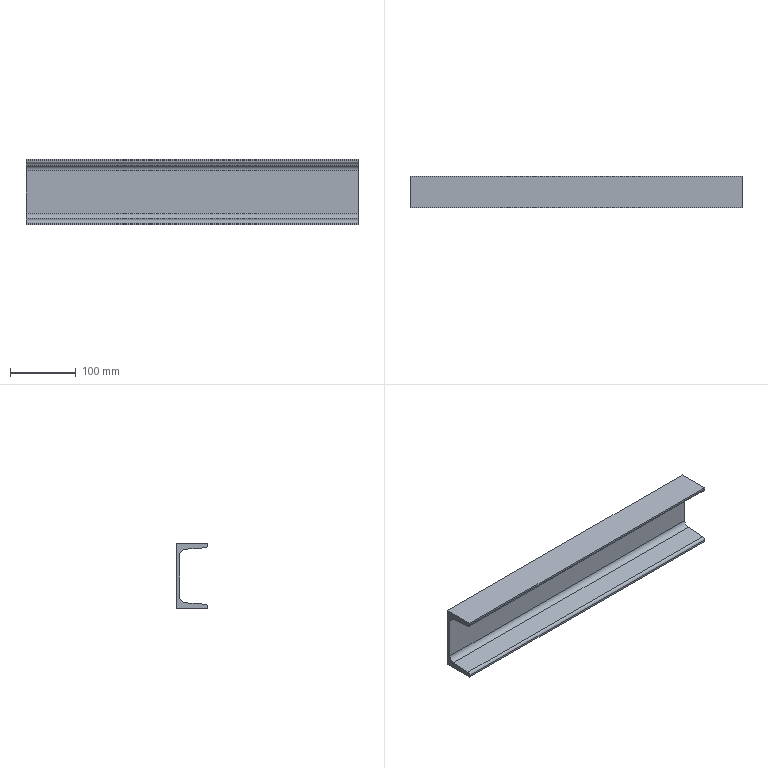Part | STEP file | 02-Channel 100x48_default<machining> | 1 solid | 14 faces | box 505 x 48 x 100 mm | volume 635347 mm3 | plane 10 | cylinder 4 | commonest cylinder face diameters 8.5 x2 17 x2
STEP:
#1=CARTESIAN_POINT('',(0.,0.,0.));
#2=DIRECTION('',(0.,0.,1.));
#3=DIRECTION('',(1.,0.,0.));
#4=AXIS2_PLACEMENT_3D('',#1,#2,#3);
#5=CARTESIAN_POINT('',(0.,-48.,-100.));
#6=VERTEX_POINT('',#5);
#7=CARTESIAN_POINT('',(0.,0.,-100.));
#8=VERTEX_POINT('',#7);
#9=CARTESIAN_POINT('',(0.,0.,-100.));
#10=DIRECTION('',(0.,1.,0.));
#11=VECTOR('',#10,1.);
#12=LINE('',#9,#11);
#13=CARTESIAN_POINT('',(505.,0.,-100.));
#14=DIRECTION('',(0.,0.,1.));
#15=DIRECTION('',(1.,0.,0.));
#16=AXIS2_PLACEMENT_3D('',#13,#14,#15);
#17=PLANE('',#16);
#18=CARTESIAN_POINT('',(-505.,0.));
#19=DIRECTION('',(0.,1.));
#20=VECTOR('',#19,1.);
#21=LINE('',#18,#20);
#22=(GEOMETRIC_REPRESENTATION_CONTEXT(2)PARAMETRIC_REPRESENTATION_CONTEXT()REPRESENTATION_CONTEXT('',''));
#23=DEFINITIONAL_REPRESENTATION('',(#21),#22);
#24=PCURVE('',#17,#23);
#25=CARTESIAN_POINT('',(0.,-43.75,-97.266));
#26=DIRECTION('',(1.,0.,0.));
#27=DIRECTION('',(0.,0.,-1.));
#28=AXIS2_PLACEMENT_3D('',#25,#26,#27);
#29=PLANE('',#28);
#30=CARTESIAN_POINT('',(2.734,43.75));
#31=DIRECTION('',(0.,1.));
#32=VECTOR('',#31,1.);
#33=LINE('',#30,#32);
#34=(GEOMETRIC_REPRESENTATION_CONTEXT(2)PARAMETRIC_REPRESENTATION_CONTEXT()REPRESENTATION_CONTEXT('',''));
#35=DEFINITIONAL_REPRESENTATION('',(#33),#34);
#36=PCURVE('',#29,#35);
#37=SURFACE_CURVE('',#12,(#24,#36),.PCURVE_S1.);
#38=EDGE_CURVE('',#6,#8,#37,.T.);
#39=ORIENTED_EDGE('',*,*,#38,.T.);
#40=CARTESIAN_POINT('',(505.,0.,-100.));
#41=VERTEX_POINT('',#40);
#42=CARTESIAN_POINT('',(505.,0.,-100.));
#43=DIRECTION('',(-1.,0.,0.));
#44=VECTOR('',#43,1.);
#45=LINE('',#42,#44);
#46=CARTESIAN_POINT('',(0.,0.));
#47=DIRECTION('',(-1.,0.));
#48=VECTOR('',#47,1.);
#49=LINE('',#46,#48);
#50=(GEOMETRIC_REPRESENTATION_CONTEXT(2)PARAMETRIC_REPRESENTATION_CONTEXT()REPRESENTATION_CONTEXT('',''));
#51=DEFINITIONAL_REPRESENTATION('',(#49),#50);
#52=PCURVE('',#17,#51);
#53=CARTESIAN_POINT('',(505.,0.,0.));
#54=DIRECTION('',(0.,-1.,0.));
#55=DIRECTION('',(0.,0.,-1.));
#56=AXIS2_PLACEMENT_3D('',#53,#54,#55);
#57=PLANE('',#56);
#58=CARTESIAN_POINT('',(100.,0.));
#59=DIRECTION('',(0.,-1.));
#60=VECTOR('',#59,1.);
#61=LINE('',#58,#60);
#62=(GEOMETRIC_REPRESENTATION_CONTEXT(2)PARAMETRIC_REPRESENTATION_CONTEXT()REPRESENTATION_CONTEXT('',''));
#63=DEFINITIONAL_REPRESENTATION('',(#61),#62);
#64=PCURVE('',#57,#63);
#65=SURFACE_CURVE('',#45,(#52,#64),.PCURVE_S1.);
#66=EDGE_CURVE('',#41,#8,#65,.T.);
#67=ORIENTED_EDGE('',*,*,#66,.F.);
#68=CARTESIAN_POINT('',(505.,-48.,-100.));
#69=VERTEX_POINT('',#68);
#70=CARTESIAN_POINT('',(505.,0.,-100.));
#71=DIRECTION('',(0.,1.,0.));
#72=VECTOR('',#71,1.);
#73=LINE('',#70,#72);
#74=CARTESIAN_POINT('',(0.,0.));
#75=DIRECTION('',(0.,1.));
#76=VECTOR('',#75,1.);
#77=LINE('',#74,#76);
#78=(GEOMETRIC_REPRESENTATION_CONTEXT(2)PARAMETRIC_REPRESENTATION_CONTEXT()REPRESENTATION_CONTEXT('',''));
#79=DEFINITIONAL_REPRESENTATION('',(#77),#78);
#80=PCURVE('',#17,#79);
#81=CARTESIAN_POINT('',(505.,-43.75,-97.266));
#82=DIRECTION('',(1.,0.,0.));
#83=DIRECTION('',(0.,0.,-1.));
#84=AXIS2_PLACEMENT_3D('',#81,#82,#83);
#85=PLANE('',#84);
#86=CARTESIAN_POINT('',(2.734,43.75));
#87=DIRECTION('',(0.,1.));
#88=VECTOR('',#87,1.);
#89=LINE('',#86,#88);
#90=(GEOMETRIC_REPRESENTATION_CONTEXT(2)PARAMETRIC_REPRESENTATION_CONTEXT()REPRESENTATION_CONTEXT('',''));
#91=DEFINITIONAL_REPRESENTATION('',(#89),#90);
#92=PCURVE('',#85,#91);
#93=SURFACE_CURVE('',#73,(#80,#92),.PCURVE_S1.);
#94=EDGE_CURVE('',#69,#41,#93,.T.);
#95=ORIENTED_EDGE('',*,*,#94,.F.);
#96=CARTESIAN_POINT('',(505.,-48.,-100.));
#97=DIRECTION('',(-1.,0.,0.));
#98=VECTOR('',#97,1.);
#99=LINE('',#96,#98);
#100=CARTESIAN_POINT('',(0.,-48.));
#101=DIRECTION('',(-1.,0.));
#102=VECTOR('',#101,1.);
#103=LINE('',#100,#102);
#104=(GEOMETRIC_REPRESENTATION_CONTEXT(2)PARAMETRIC_REPRESENTATION_CONTEXT()REPRESENTATION_CONTEXT('',''));
#105=DEFINITIONAL_REPRESENTATION('',(#103),#104);
#106=PCURVE('',#17,#105);
#107=CARTESIAN_POINT('',(505.,-48.,-97.266));
#108=DIRECTION('',(0.,1.,0.));
#109=DIRECTION('',(0.,0.,1.));
#110=AXIS2_PLACEMENT_3D('',#107,#108,#109);
#111=PLANE('',#110);
#112=CARTESIAN_POINT('',(-2.734,0.));
#113=DIRECTION('',(0.,-1.));
#114=VECTOR('',#113,1.);
#115=LINE('',#112,#114);
#116=(GEOMETRIC_REPRESENTATION_CONTEXT(2)PARAMETRIC_REPRESENTATION_CONTEXT()REPRESENTATION_CONTEXT('',''));
#117=DEFINITIONAL_REPRESENTATION('',(#115),#116);
#118=PCURVE('',#111,#117);
#119=SURFACE_CURVE('',#99,(#106,#118),.PCURVE_S1.);
#120=EDGE_CURVE('',#69,#6,#119,.T.);
#121=ORIENTED_EDGE('',*,*,#120,.T.);
#122=EDGE_LOOP('',(#39,#67,#95,#121));
#123=FACE_BOUND('',#122,.T.);
#124=ADVANCED_FACE('',(#123),#17,.F.);
#125=CARTESIAN_POINT('',(0.,0.,0.));
#126=VERTEX_POINT('',#125);
#127=CARTESIAN_POINT('',(0.,0.,0.));
#128=DIRECTION('',(0.,0.,1.));
#129=VECTOR('',#128,1.);
#130=LINE('',#127,#129);
#131=CARTESIAN_POINT('',(0.,-505.));
#132=DIRECTION('',(-1.,0.));
#133=VECTOR('',#132,1.);
#134=LINE('',#131,#133);
#135=(GEOMETRIC_REPRESENTATION_CONTEXT(2)PARAMETRIC_REPRESENTATION_CONTEXT()REPRESENTATION_CONTEXT('',''));
#136=DEFINITIONAL_REPRESENTATION('',(#134),#135);
#137=PCURVE('',#57,#136);
#138=CARTESIAN_POINT('',(-97.266,43.75));
#139=DIRECTION('',(-1.,0.));
#140=VECTOR('',#139,1.);
#141=LINE('',#138,#140);
#142=(GEOMETRIC_REPRESENTATION_CONTEXT(2)PARAMETRIC_REPRESENTATION_CONTEXT()REPRESENTATION_CONTEXT('',''));
#143=DEFINITIONAL_REPRESENTATION('',(#141),#142);
#144=PCURVE('',#29,#143);
#145=SURFACE_CURVE('',#130,(#137,#144),.PCURVE_S1.);
#146=EDGE_CURVE('',#8,#126,#145,.T.);
#147=ORIENTED_EDGE('',*,*,#146,.T.);
#148=CARTESIAN_POINT('',(505.,0.,0.));
#149=VERTEX_POINT('',#148);
#150=CARTESIAN_POINT('',(505.,0.,0.));
#151=DIRECTION('',(-1.,0.,0.));
#152=VECTOR('',#151,1.);
#153=LINE('',#150,#152);
#154=CARTESIAN_POINT('',(0.,0.));
#155=DIRECTION('',(0.,-1.));
#156=VECTOR('',#155,1.);
#157=LINE('',#154,#156);
#158=(GEOMETRIC_REPRESENTATION_CONTEXT(2)PARAMETRIC_REPRESENTATION_CONTEXT()REPRESENTATION_CONTEXT('',''));
#159=DEFINITIONAL_REPRESENTATION('',(#157),#158);
#160=PCURVE('',#57,#159);
#161=CARTESIAN_POINT('',(505.,0.,0.));
#162=DIRECTION('',(0.,0.,-1.));
#163=DIRECTION('',(0.,1.,0.));
#164=AXIS2_PLACEMENT_3D('',#161,#162,#163);
#165=PLANE('',#164);
#166=CARTESIAN_POINT('',(0.,0.));
#167=DIRECTION('',(0.,-1.));
#168=VECTOR('',#167,1.);
#169=LINE('',#166,#168);
#170=(GEOMETRIC_REPRESENTATION_CONTEXT(2)PARAMETRIC_REPRESENTATION_CONTEXT()REPRESENTATION_CONTEXT('',''));
#171=DEFINITIONAL_REPRESENTATION('',(#169),#170);
#172=PCURVE('',#165,#171);
#173=SURFACE_CURVE('',#153,(#160,#172),.PCURVE_S1.);
#174=EDGE_CURVE('',#149,#126,#173,.T.);
#175=ORIENTED_EDGE('',*,*,#174,.F.);
#176=CARTESIAN_POINT('',(505.,0.,0.));
#177=DIRECTION('',(0.,0.,1.));
#178=VECTOR('',#177,1.);
#179=LINE('',#176,#178);
#180=CARTESIAN_POINT('',(0.,0.));
#181=DIRECTION('',(-1.,0.));
#182=VECTOR('',#181,1.);
#183=LINE('',#180,#182);
#184=(GEOMETRIC_REPRESENTATION_CONTEXT(2)PARAMETRIC_REPRESENTATION_CONTEXT()REPRESENTATION_CONTEXT('',''));
#185=DEFINITIONAL_REPRESENTATION('',(#183),#184);
#186=PCURVE('',#57,#185);
#187=CARTESIAN_POINT('',(-97.266,43.75));
#188=DIRECTION('',(-1.,0.));
#189=VECTOR('',#188,1.);
#190=LINE('',#187,#189);
#191=(GEOMETRIC_REPRESENTATION_CONTEXT(2)PARAMETRIC_REPRESENTATION_CONTEXT()REPRESENTATION_CONTEXT('',''));
#192=DEFINITIONAL_REPRESENTATION('',(#190),#191);
#193=PCURVE('',#85,#192);
#194=SURFACE_CURVE('',#179,(#186,#193),.PCURVE_S1.);
#195=EDGE_CURVE('',#41,#149,#194,.T.);
#196=ORIENTED_EDGE('',*,*,#195,.F.);
#197=ORIENTED_EDGE('',*,*,#66,.T.);
#198=EDGE_LOOP('',(#147,#175,#196,#197));
#199=FACE_BOUND('',#198,.T.);
#200=ADVANCED_FACE('',(#199),#57,.F.);
#201=CARTESIAN_POINT('',(0.,-48.,0.));
#202=VERTEX_POINT('',#201);
#203=CARTESIAN_POINT('',(0.,0.,0.));
#204=DIRECTION('',(0.,-1.,0.));
#205=VECTOR('',#204,1.);
#206=LINE('',#203,#205);
#207=CARTESIAN_POINT('',(0.,-505.));
#208=DIRECTION('',(-1.,0.));
#209=VECTOR('',#208,1.);
#210=LINE('',#207,#209);
#211=(GEOMETRIC_REPRESENTATION_CONTEXT(2)PARAMETRIC_REPRESENTATION_CONTEXT()REPRESENTATION_CONTEXT('',''));
#212=DEFINITIONAL_REPRESENTATION('',(#210),#211);
#213=PCURVE('',#165,#212);
#214=CARTESIAN_POINT('',(-97.266,43.75));
#215=DIRECTION('',(0.,-1.));
#216=VECTOR('',#215,1.);
#217=LINE('',#214,#216);
#218=(GEOMETRIC_REPRESENTATION_CONTEXT(2)PARAMETRIC_REPRESENTATION_CONTEXT()REPRESENTATION_CONTEXT('',''));
#219=DEFINITIONAL_REPRESENTATION('',(#217),#218);
#220=PCURVE('',#29,#219);
#221=SURFACE_CURVE('',#206,(#213,#220),.PCURVE_S1.);
#222=EDGE_CURVE('',#126,#202,#221,.T.);
#223=ORIENTED_EDGE('',*,*,#222,.T.);
#224=CARTESIAN_POINT('',(505.,-48.,0.));
#225=VERTEX_POINT('',#224);
#226=CARTESIAN_POINT('',(505.,-48.,0.));
#227=DIRECTION('',(-1.,0.,0.));
#228=VECTOR('',#227,1.);
#229=LINE('',#226,#228);
#230=CARTESIAN_POINT('',(-48.,0.));
#231=DIRECTION('',(0.,-1.));
#232=VECTOR('',#231,1.);
#233=LINE('',#230,#232);
#234=(GEOMETRIC_REPRESENTATION_CONTEXT(2)PARAMETRIC_REPRESENTATION_CONTEXT()REPRESENTATION_CONTEXT('',''));
#235=DEFINITIONAL_REPRESENTATION('',(#233),#234);
#236=PCURVE('',#165,#235);
#237=CARTESIAN_POINT('',(505.,-48.,-2.734));
#238=DIRECTION('',(0.,1.,0.));
#239=DIRECTION('',(0.,0.,1.));
#240=AXIS2_PLACEMENT_3D('',#237,#238,#239);
#241=PLANE('',#240);
#242=CARTESIAN_POINT('',(2.734,0.));
#243=DIRECTION('',(0.,-1.));
#244=VECTOR('',#243,1.);
#245=LINE('',#242,#244);
#246=(GEOMETRIC_REPRESENTATION_CONTEXT(2)PARAMETRIC_REPRESENTATION_CONTEXT()REPRESENTATION_CONTEXT('',''));
#247=DEFINITIONAL_REPRESENTATION('',(#245),#246);
#248=PCURVE('',#241,#247);
#249=SURFACE_CURVE('',#229,(#236,#248),.PCURVE_S1.);
#250=EDGE_CURVE('',#225,#202,#249,.T.);
#251=ORIENTED_EDGE('',*,*,#250,.F.);
#252=CARTESIAN_POINT('',(505.,0.,0.));
#253=DIRECTION('',(0.,-1.,0.));
#254=VECTOR('',#253,1.);
#255=LINE('',#252,#254);
#256=CARTESIAN_POINT('',(0.,0.));
#257=DIRECTION('',(-1.,0.));
#258=VECTOR('',#257,1.);
#259=LINE('',#256,#258);
#260=(GEOMETRIC_REPRESENTATION_CONTEXT(2)PARAMETRIC_REPRESENTATION_CONTEXT()REPRESENTATION_CONTEXT('',''));
#261=DEFINITIONAL_REPRESENTATION('',(#259),#260);
#262=PCURVE('',#165,#261);
#263=CARTESIAN_POINT('',(-97.266,43.75));
#264=DIRECTION('',(0.,-1.));
#265=VECTOR('',#264,1.);
#266=LINE('',#263,#265);
#267=(GEOMETRIC_REPRESENTATION_CONTEXT(2)PARAMETRIC_REPRESENTATION_CONTEXT()REPRESENTATION_CONTEXT('',''));
#268=DEFINITIONAL_REPRESENTATION('',(#266),#267);
#269=PCURVE('',#85,#268);
#270=SURFACE_CURVE('',#255,(#262,#269),.PCURVE_S1.);
#271=EDGE_CURVE('',#149,#225,#270,.T.);
#272=ORIENTED_EDGE('',*,*,#271,.F.);
#273=ORIENTED_EDGE('',*,*,#174,.T.);
#274=EDGE_LOOP('',(#223,#251,#272,#273));
#275=FACE_BOUND('',#274,.T.);
#276=ADVANCED_FACE('',(#275),#165,.F.);
#277=CARTESIAN_POINT('',(0.,-48.,-2.734));
#278=VERTEX_POINT('',#277);
#279=CARTESIAN_POINT('',(0.,-48.,-2.734));
#280=DIRECTION('',(0.,0.,-1.));
#281=VECTOR('',#280,1.);
#282=LINE('',#279,#281);
#283=CARTESIAN_POINT('',(0.,-505.));
#284=DIRECTION('',(-1.,0.));
#285=VECTOR('',#284,1.);
#286=LINE('',#283,#285);
#287=(GEOMETRIC_REPRESENTATION_CONTEXT(2)PARAMETRIC_REPRESENTATION_CONTEXT()REPRESENTATION_CONTEXT('',''));
#288=DEFINITIONAL_REPRESENTATION('',(#286),#287);
#289=PCURVE('',#241,#288);
#290=CARTESIAN_POINT('',(-94.531,-4.25));
#291=DIRECTION('',(1.,0.));
#292=VECTOR('',#291,1.);
#293=LINE('',#290,#292);
#294=(GEOMETRIC_REPRESENTATION_CONTEXT(2)PARAMETRIC_REPRESENTATION_CONTEXT()REPRESENTATION_CONTEXT('',''));
#295=DEFINITIONAL_REPRESENTATION('',(#293),#294);
#296=PCURVE('',#29,#295);
#297=SURFACE_CURVE('',#282,(#289,#296),.PCURVE_S1.);
#298=EDGE_CURVE('',#202,#278,#297,.T.);
#299=ORIENTED_EDGE('',*,*,#298,.T.);
#300=CARTESIAN_POINT('',(505.,-48.,-2.734));
#301=VERTEX_POINT('',#300);
#302=CARTESIAN_POINT('',(505.,-48.,-2.734));
#303=DIRECTION('',(-1.,0.,0.));
#304=VECTOR('',#303,1.);
#305=LINE('',#302,#304);
#306=CARTESIAN_POINT('',(0.,0.));
#307=DIRECTION('',(0.,-1.));
#308=VECTOR('',#307,1.);
#309=LINE('',#306,#308);
#310=(GEOMETRIC_REPRESENTATION_CONTEXT(2)PARAMETRIC_REPRESENTATION_CONTEXT()REPRESENTATION_CONTEXT('',''));
#311=DEFINITIONAL_REPRESENTATION('',(#309),#310);
#312=PCURVE('',#241,#311);
#313=CARTESIAN_POINT('',(505.,-43.75,-2.734));
#314=DIRECTION('',(-1.,0.,0.));
#315=DIRECTION('',(0.,0.,1.));
#316=AXIS2_PLACEMENT_3D('',#313,#314,#315);
#317=CYLINDRICAL_SURFACE('',#316,4.25);
#318=CARTESIAN_POINT('',(4.712,0.));
#319=DIRECTION('',(0.,1.));
#320=VECTOR('',#319,1.);
#321=LINE('',#318,#320);
#322=(GEOMETRIC_REPRESENTATION_CONTEXT(2)PARAMETRIC_REPRESENTATION_CONTEXT()REPRESENTATION_CONTEXT('',''));
#323=DEFINITIONAL_REPRESENTATION('',(#321),#322);
#324=PCURVE('',#317,#323);
#325=SURFACE_CURVE('',#305,(#312,#324),.PCURVE_S1.);
#326=EDGE_CURVE('',#301,#278,#325,.T.);
#327=ORIENTED_EDGE('',*,*,#326,.F.);
#328=CARTESIAN_POINT('',(505.,-48.,-2.734));
#329=DIRECTION('',(0.,0.,-1.));
#330=VECTOR('',#329,1.);
#331=LINE('',#328,#330);
#332=CARTESIAN_POINT('',(0.,0.));
#333=DIRECTION('',(-1.,0.));
#334=VECTOR('',#333,1.);
#335=LINE('',#332,#334);
#336=(GEOMETRIC_REPRESENTATION_CONTEXT(2)PARAMETRIC_REPRESENTATION_CONTEXT()REPRESENTATION_CONTEXT('',''));
#337=DEFINITIONAL_REPRESENTATION('',(#335),#336);
#338=PCURVE('',#241,#337);
#339=CARTESIAN_POINT('',(-94.531,-4.25));
#340=DIRECTION('',(1.,0.));
#341=VECTOR('',#340,1.);
#342=LINE('',#339,#341);
#343=(GEOMETRIC_REPRESENTATION_CONTEXT(2)PARAMETRIC_REPRESENTATION_CONTEXT()REPRESENTATION_CONTEXT('',''));
#344=DEFINITIONAL_REPRESENTATION('',(#342),#343);
#345=PCURVE('',#85,#344);
#346=SURFACE_CURVE('',#331,(#338,#345),.PCURVE_S1.);
#347=EDGE_CURVE('',#225,#301,#346,.T.);
#348=ORIENTED_EDGE('',*,*,#347,.F.);
#349=ORIENTED_EDGE('',*,*,#250,.T.);
#350=EDGE_LOOP('',(#299,#327,#348,#349));
#351=FACE_BOUND('',#350,.T.);
#352=ADVANCED_FACE('',(#351),#241,.F.);
#353=CARTESIAN_POINT('',(0.,-44.073,-6.972));
#354=VERTEX_POINT('',#353);
#355=CARTESIAN_POINT('',(0.,-43.75,-2.734));
#356=DIRECTION('',(1.,0.,0.));
#357=DIRECTION('',(0.,0.,-1.));
#358=AXIS2_PLACEMENT_3D('',#355,#356,#357);
#359=CIRCLE('',#358,4.25);
#360=CARTESIAN_POINT('',(9.425,505.));
#361=DIRECTION('',(-1.,0.));
#362=VECTOR('',#361,1.);
#363=LINE('',#360,#362);
#364=(GEOMETRIC_REPRESENTATION_CONTEXT(2)PARAMETRIC_REPRESENTATION_CONTEXT()REPRESENTATION_CONTEXT('',''));
#365=DEFINITIONAL_REPRESENTATION('',(#363),#364);
#366=PCURVE('',#317,#365);
#367=CARTESIAN_POINT('',(-94.531,0.));
#368=DIRECTION('',(1.,0.));
#369=AXIS2_PLACEMENT_2D('',#367,#368);
#370=CIRCLE('',#369,4.25);
#371=(GEOMETRIC_REPRESENTATION_CONTEXT(2)PARAMETRIC_REPRESENTATION_CONTEXT()REPRESENTATION_CONTEXT('',''));
#372=DEFINITIONAL_REPRESENTATION('',(#370),#371);
#373=PCURVE('',#29,#372);
#374=SURFACE_CURVE('',#359,(#366,#373),.PCURVE_S1.);
#375=EDGE_CURVE('',#278,#354,#374,.T.);
#376=ORIENTED_EDGE('',*,*,#375,.T.);
#377=CARTESIAN_POINT('',(505.,-44.073,-6.972));
#378=VERTEX_POINT('',#377);
#379=CARTESIAN_POINT('',(505.,-44.073,-6.972));
#380=DIRECTION('',(-1.,0.,0.));
#381=VECTOR('',#380,1.);
#382=LINE('',#379,#381);
#383=CARTESIAN_POINT('',(3.218,0.));
#384=DIRECTION('',(0.,1.));
#385=VECTOR('',#384,1.);
#386=LINE('',#383,#385);
#387=(GEOMETRIC_REPRESENTATION_CONTEXT(2)PARAMETRIC_REPRESENTATION_CONTEXT()REPRESENTATION_CONTEXT('',''));
#388=DEFINITIONAL_REPRESENTATION('',(#386),#387);
#389=PCURVE('',#317,#388);
#390=CARTESIAN_POINT('',(505.,-13.155,-9.325));
#391=DIRECTION('',(0.,0.07589,0.9971));
#392=DIRECTION('',(0.,-0.9971,0.07589));
#393=AXIS2_PLACEMENT_3D('',#390,#391,#392);
#394=PLANE('',#393);
#395=CARTESIAN_POINT('',(31.007,0.));
#396=DIRECTION('',(0.,-1.));
#397=VECTOR('',#396,1.);
#398=LINE('',#395,#397);
#399=(GEOMETRIC_REPRESENTATION_CONTEXT(2)PARAMETRIC_REPRESENTATION_CONTEXT()REPRESENTATION_CONTEXT('',''));
#400=DEFINITIONAL_REPRESENTATION('',(#398),#399);
#401=PCURVE('',#394,#400);
#402=SURFACE_CURVE('',#382,(#389,#401),.PCURVE_S1.);
#403=EDGE_CURVE('',#378,#354,#402,.T.);
#404=ORIENTED_EDGE('',*,*,#403,.F.);
#405=CARTESIAN_POINT('',(505.,-43.75,-2.734));
#406=DIRECTION('',(1.,0.,0.));
#407=DIRECTION('',(0.,0.,-1.));
#408=AXIS2_PLACEMENT_3D('',#405,#406,#407);
#409=CIRCLE('',#408,4.25);
#410=CARTESIAN_POINT('',(9.425,0.));
#411=DIRECTION('',(-1.,0.));
#412=VECTOR('',#411,1.);
#413=LINE('',#410,#412);
#414=(GEOMETRIC_REPRESENTATION_CONTEXT(2)PARAMETRIC_REPRESENTATION_CONTEXT()REPRESENTATION_CONTEXT('',''));
#415=DEFINITIONAL_REPRESENTATION('',(#413),#414);
#416=PCURVE('',#317,#415);
#417=CARTESIAN_POINT('',(-94.531,0.));
#418=DIRECTION('',(1.,0.));
#419=AXIS2_PLACEMENT_2D('',#417,#418);
#420=CIRCLE('',#419,4.25);
#421=(GEOMETRIC_REPRESENTATION_CONTEXT(2)PARAMETRIC_REPRESENTATION_CONTEXT()REPRESENTATION_CONTEXT('',''));
#422=DEFINITIONAL_REPRESENTATION('',(#420),#421);
#423=PCURVE('',#85,#422);
#424=SURFACE_CURVE('',#409,(#416,#423),.PCURVE_S1.);
#425=EDGE_CURVE('',#301,#378,#424,.T.);
#426=ORIENTED_EDGE('',*,*,#425,.F.);
#427=ORIENTED_EDGE('',*,*,#326,.T.);
#428=EDGE_LOOP('',(#376,#404,#426,#427));
#429=FACE_BOUND('',#428,.T.);
#430=ADVANCED_FACE('',(#429),#317,.T.);
#431=CARTESIAN_POINT('',(0.,-13.155,-9.325));
#432=VERTEX_POINT('',#431);
#433=CARTESIAN_POINT('',(0.,-13.155,-9.325));
#434=DIRECTION('',(0.,0.9971,-0.07589));
#435=VECTOR('',#434,1.);
#436=LINE('',#433,#435);
#437=CARTESIAN_POINT('',(0.,-505.));
#438=DIRECTION('',(-1.,0.));
#439=VECTOR('',#438,1.);
#440=LINE('',#437,#439);
#441=(GEOMETRIC_REPRESENTATION_CONTEXT(2)PARAMETRIC_REPRESENTATION_CONTEXT()REPRESENTATION_CONTEXT('',''));
#442=DEFINITIONAL_REPRESENTATION('',(#440),#441);
#443=PCURVE('',#394,#442);
#444=CARTESIAN_POINT('',(-87.94,30.595));
#445=DIRECTION('',(0.07589,0.9971));
#446=VECTOR('',#445,1.);
#447=LINE('',#444,#446);
#448=(GEOMETRIC_REPRESENTATION_CONTEXT(2)PARAMETRIC_REPRESENTATION_CONTEXT()REPRESENTATION_CONTEXT('',''));
#449=DEFINITIONAL_REPRESENTATION('',(#447),#448);
#450=PCURVE('',#29,#449);
#451=SURFACE_CURVE('',#436,(#443,#450),.PCURVE_S1.);
#452=EDGE_CURVE('',#354,#432,#451,.T.);
#453=ORIENTED_EDGE('',*,*,#452,.T.);
#454=CARTESIAN_POINT('',(505.,-13.155,-9.325));
#455=VERTEX_POINT('',#454);
#456=CARTESIAN_POINT('',(505.,-13.155,-9.325));
#457=DIRECTION('',(-1.,0.,0.));
#458=VECTOR('',#457,1.);
#459=LINE('',#456,#458);
#460=CARTESIAN_POINT('',(0.,0.));
#461=DIRECTION('',(0.,-1.));
#462=VECTOR('',#461,1.);
#463=LINE('',#460,#462);
#464=(GEOMETRIC_REPRESENTATION_CONTEXT(2)PARAMETRIC_REPRESENTATION_CONTEXT()REPRESENTATION_CONTEXT('',''));
#465=DEFINITIONAL_REPRESENTATION('',(#463),#464);
#466=PCURVE('',#394,#465);
#467=CARTESIAN_POINT('',(505.,-13.8,-17.801));
#468=DIRECTION('',(-1.,0.,0.));
#469=DIRECTION('',(0.,0.,1.));
#470=AXIS2_PLACEMENT_3D('',#467,#468,#469);
#471=CYLINDRICAL_SURFACE('',#470,8.5);
#472=CARTESIAN_POINT('',(0.07597,0.));
#473=DIRECTION('',(0.,1.));
#474=VECTOR('',#473,1.);
#475=LINE('',#472,#474);
#476=(GEOMETRIC_REPRESENTATION_CONTEXT(2)PARAMETRIC_REPRESENTATION_CONTEXT()REPRESENTATION_CONTEXT('',''));
#477=DEFINITIONAL_REPRESENTATION('',(#475),#476);
#478=PCURVE('',#471,#477);
#479=SURFACE_CURVE('',#459,(#466,#478),.PCURVE_S1.);
#480=EDGE_CURVE('',#455,#432,#479,.T.);
#481=ORIENTED_EDGE('',*,*,#480,.F.);
#482=CARTESIAN_POINT('',(505.,-13.155,-9.325));
#483=DIRECTION('',(0.,0.9971,-0.07589));
#484=VECTOR('',#483,1.);
#485=LINE('',#482,#484);
#486=CARTESIAN_POINT('',(0.,0.));
#487=DIRECTION('',(-1.,0.));
#488=VECTOR('',#487,1.);
#489=LINE('',#486,#488);
#490=(GEOMETRIC_REPRESENTATION_CONTEXT(2)PARAMETRIC_REPRESENTATION_CONTEXT()REPRESENTATION_CONTEXT('',''));
#491=DEFINITIONAL_REPRESENTATION('',(#489),#490);
#492=PCURVE('',#394,#491);
#493=CARTESIAN_POINT('',(-87.94,30.595));
#494=DIRECTION('',(0.07589,0.9971));
#495=VECTOR('',#494,1.);
#496=LINE('',#493,#495);
#497=(GEOMETRIC_REPRESENTATION_CONTEXT(2)PARAMETRIC_REPRESENTATION_CONTEXT()REPRESENTATION_CONTEXT('',''));
#498=DEFINITIONAL_REPRESENTATION('',(#496),#497);
#499=PCURVE('',#85,#498);
#500=SURFACE_CURVE('',#485,(#492,#499),.PCURVE_S1.);
#501=EDGE_CURVE('',#378,#455,#500,.T.);
#502=ORIENTED_EDGE('',*,*,#501,.F.);
#503=ORIENTED_EDGE('',*,*,#403,.T.);
#504=EDGE_LOOP('',(#453,#481,#502,#503));
#505=FACE_BOUND('',#504,.T.);
#506=ADVANCED_FACE('',(#505),#394,.F.);
#507=ORIENTED_EDGE('',*,*,#480,.F.);
#508=CARTESIAN_POINT('',(505.,-5.3,-17.801));
#509=VERTEX_POINT('',#508);
#510=CARTESIAN_POINT('',(505.,-13.8,-17.801));
#511=DIRECTION('',(-1.,0.,0.));
#512=DIRECTION('',(0.,0.,1.));
#513=AXIS2_PLACEMENT_3D('',#510,#511,#512);
#514=CIRCLE('',#513,8.5);
#515=CARTESIAN_POINT('',(0.,0.));
#516=DIRECTION('',(1.,0.));
#517=VECTOR('',#516,1.);
#518=LINE('',#515,#517);
#519=(GEOMETRIC_REPRESENTATION_CONTEXT(2)PARAMETRIC_REPRESENTATION_CONTEXT()REPRESENTATION_CONTEXT('',''));
#520=DEFINITIONAL_REPRESENTATION('',(#518),#519);
#521=PCURVE('',#471,#520);
#522=CARTESIAN_POINT('',(-87.965,29.95));
#523=CARTESIAN_POINT('',(-87.965,44.672));
#524=CARTESIAN_POINT('',(-75.215,37.311));
#525=CARTESIAN_POINT('',(-62.465,29.95));
#526=CARTESIAN_POINT('',(-75.215,22.589));
#527=CARTESIAN_POINT('',(-87.965,15.228));
#528=CARTESIAN_POINT('',(-87.965,29.95));
#529=(BOUNDED_CURVE()B_SPLINE_CURVE(2,(#522,#523,#524,#525,#526,#527,#528),.UNSPECIFIED.,.T.,.F.)B_SPLINE_CURVE_WITH_KNOTS((1,2,2,2,2,1),(-2.094,0.,2.094,4.189,6.283,8.378),.UNSPECIFIED.)CURVE()GEOMETRIC_REPRESENTATION_ITEM()RATIONAL_B_SPLINE_CURVE((1.,0.5,1.,0.5,1.,0.5,1.))REPRESENTATION_ITEM(''));
#530=(GEOMETRIC_REPRESENTATION_CONTEXT(2)PARAMETRIC_REPRESENTATION_CONTEXT()REPRESENTATION_CONTEXT('',''));
#531=DEFINITIONAL_REPRESENTATION('',(#529),#530);
#532=PCURVE('',#85,#531);
#533=SURFACE_CURVE('',#514,(#521,#532),.PCURVE_S1.);
#534=EDGE_CURVE('',#455,#509,#533,.T.);
#535=ORIENTED_EDGE('',*,*,#534,.T.);
#536=CARTESIAN_POINT('',(0.,-5.3,-17.801));
#537=VERTEX_POINT('',#536);
#538=CARTESIAN_POINT('',(505.,-5.3,-17.801));
#539=DIRECTION('',(-1.,0.,0.));
#540=VECTOR('',#539,1.);
#541=LINE('',#538,#540);
#542=CARTESIAN_POINT('',(1.571,0.));
#543=DIRECTION('',(0.,1.));
#544=VECTOR('',#543,1.);
#545=LINE('',#542,#544);
#546=(GEOMETRIC_REPRESENTATION_CONTEXT(2)PARAMETRIC_REPRESENTATION_CONTEXT()REPRESENTATION_CONTEXT('',''));
#547=DEFINITIONAL_REPRESENTATION('',(#545),#546);
#548=PCURVE('',#471,#547);
#549=CARTESIAN_POINT('',(505.,-5.3,-82.199));
#550=DIRECTION('',(0.,1.,0.));
#551=DIRECTION('',(0.,0.,1.));
#552=AXIS2_PLACEMENT_3D('',#549,#550,#551);
#553=PLANE('',#552);
#554=CARTESIAN_POINT('',(64.398,0.));
#555=DIRECTION('',(0.,-1.));
#556=VECTOR('',#555,1.);
#557=LINE('',#554,#556);
#558=(GEOMETRIC_REPRESENTATION_CONTEXT(2)PARAMETRIC_REPRESENTATION_CONTEXT()REPRESENTATION_CONTEXT('',''));
#559=DEFINITIONAL_REPRESENTATION('',(#557),#558);
#560=PCURVE('',#553,#559);
#561=SURFACE_CURVE('',#541,(#548,#560),.PCURVE_S1.);
#562=EDGE_CURVE('',#509,#537,#561,.T.);
#563=ORIENTED_EDGE('',*,*,#562,.T.);
#564=CARTESIAN_POINT('',(0.,-13.8,-17.801));
#565=DIRECTION('',(-1.,0.,0.));
#566=DIRECTION('',(0.,0.,1.));
#567=AXIS2_PLACEMENT_3D('',#564,#565,#566);
#568=CIRCLE('',#567,8.5);
#569=CARTESIAN_POINT('',(0.,505.));
#570=DIRECTION('',(1.,0.));
#571=VECTOR('',#570,1.);
#572=LINE('',#569,#571);
#573=(GEOMETRIC_REPRESENTATION_CONTEXT(2)PARAMETRIC_REPRESENTATION_CONTEXT()REPRESENTATION_CONTEXT('',''));
#574=DEFINITIONAL_REPRESENTATION('',(#572),#573);
#575=PCURVE('',#471,#574);
#576=CARTESIAN_POINT('',(-87.965,29.95));
#577=CARTESIAN_POINT('',(-87.965,44.672));
#578=CARTESIAN_POINT('',(-75.215,37.311));
#579=CARTESIAN_POINT('',(-62.465,29.95));
#580=CARTESIAN_POINT('',(-75.215,22.589));
#581=CARTESIAN_POINT('',(-87.965,15.228));
#582=CARTESIAN_POINT('',(-87.965,29.95));
#583=(BOUNDED_CURVE()B_SPLINE_CURVE(2,(#576,#577,#578,#579,#580,#581,#582),.UNSPECIFIED.,.T.,.F.)B_SPLINE_CURVE_WITH_KNOTS((1,2,2,2,2,1),(-2.094,0.,2.094,4.189,6.283,8.378),.UNSPECIFIED.)CURVE()GEOMETRIC_REPRESENTATION_ITEM()RATIONAL_B_SPLINE_CURVE((1.,0.5,1.,0.5,1.,0.5,1.))REPRESENTATION_ITEM(''));
#584=(GEOMETRIC_REPRESENTATION_CONTEXT(2)PARAMETRIC_REPRESENTATION_CONTEXT()REPRESENTATION_CONTEXT('',''));
#585=DEFINITIONAL_REPRESENTATION('',(#583),#584);
#586=PCURVE('',#29,#585);
#587=SURFACE_CURVE('',#568,(#575,#586),.PCURVE_S1.);
#588=EDGE_CURVE('',#432,#537,#587,.T.);
#589=ORIENTED_EDGE('',*,*,#588,.F.);
#590=EDGE_LOOP('',(#507,#535,#563,#589));
#591=FACE_BOUND('',#590,.F.);
#592=ADVANCED_FACE('',(#591),#471,.F.);
#593=CARTESIAN_POINT('',(0.,-5.3,-82.199));
#594=VERTEX_POINT('',#593);
#595=CARTESIAN_POINT('',(0.,-5.3,-82.199));
#596=DIRECTION('',(0.,0.,-1.));
#597=VECTOR('',#596,1.);
#598=LINE('',#595,#597);
#599=CARTESIAN_POINT('',(0.,-505.));
#600=DIRECTION('',(-1.,0.));
#601=VECTOR('',#600,1.);
#602=LINE('',#599,#601);
#603=(GEOMETRIC_REPRESENTATION_CONTEXT(2)PARAMETRIC_REPRESENTATION_CONTEXT()REPRESENTATION_CONTEXT('',''));
#604=DEFINITIONAL_REPRESENTATION('',(#602),#603);
#605=PCURVE('',#553,#604);
#606=CARTESIAN_POINT('',(-15.066,38.45));
#607=DIRECTION('',(1.,0.));
#608=VECTOR('',#607,1.);
#609=LINE('',#606,#608);
#610=(GEOMETRIC_REPRESENTATION_CONTEXT(2)PARAMETRIC_REPRESENTATION_CONTEXT()REPRESENTATION_CONTEXT('',''));
#611=DEFINITIONAL_REPRESENTATION('',(#609),#610);
#612=PCURVE('',#29,#611);
#613=SURFACE_CURVE('',#598,(#605,#612),.PCURVE_S1.);
#614=EDGE_CURVE('',#537,#594,#613,.T.);
#615=ORIENTED_EDGE('',*,*,#614,.T.);
#616=CARTESIAN_POINT('',(505.,-5.3,-82.199));
#617=VERTEX_POINT('',#616);
#618=CARTESIAN_POINT('',(505.,-5.3,-82.199));
#619=DIRECTION('',(-1.,0.,0.));
#620=VECTOR('',#619,1.);
#621=LINE('',#618,#620);
#622=CARTESIAN_POINT('',(0.,0.));
#623=DIRECTION('',(0.,-1.));
#624=VECTOR('',#623,1.);
#625=LINE('',#622,#624);
#626=(GEOMETRIC_REPRESENTATION_CONTEXT(2)PARAMETRIC_REPRESENTATION_CONTEXT()REPRESENTATION_CONTEXT('',''));
#627=DEFINITIONAL_REPRESENTATION('',(#625),#626);
#628=PCURVE('',#553,#627);
#629=CARTESIAN_POINT('',(505.,-13.8,-82.199));
#630=DIRECTION('',(-1.,0.,0.));
#631=DIRECTION('',(0.,0.,1.));
#632=AXIS2_PLACEMENT_3D('',#629,#630,#631);
#633=CYLINDRICAL_SURFACE('',#632,8.5);
#634=CARTESIAN_POINT('',(1.571,0.));
#635=DIRECTION('',(0.,1.));
#636=VECTOR('',#635,1.);
#637=LINE('',#634,#636);
#638=(GEOMETRIC_REPRESENTATION_CONTEXT(2)PARAMETRIC_REPRESENTATION_CONTEXT()REPRESENTATION_CONTEXT('',''));
#639=DEFINITIONAL_REPRESENTATION('',(#637),#638);
#640=PCURVE('',#633,#639);
#641=SURFACE_CURVE('',#621,(#628,#640),.PCURVE_S1.);
#642=EDGE_CURVE('',#617,#594,#641,.T.);
#643=ORIENTED_EDGE('',*,*,#642,.F.);
#644=CARTESIAN_POINT('',(505.,-5.3,-82.199));
#645=DIRECTION('',(0.,0.,-1.));
#646=VECTOR('',#645,1.);
#647=LINE('',#644,#646);
#648=CARTESIAN_POINT('',(0.,0.));
#649=DIRECTION('',(-1.,0.));
#650=VECTOR('',#649,1.);
#651=LINE('',#648,#650);
#652=(GEOMETRIC_REPRESENTATION_CONTEXT(2)PARAMETRIC_REPRESENTATION_CONTEXT()REPRESENTATION_CONTEXT('',''));
#653=DEFINITIONAL_REPRESENTATION('',(#651),#652);
#654=PCURVE('',#553,#653);
#655=CARTESIAN_POINT('',(-15.066,38.45));
#656=DIRECTION('',(1.,0.));
#657=VECTOR('',#656,1.);
#658=LINE('',#655,#657);
#659=(GEOMETRIC_REPRESENTATION_CONTEXT(2)PARAMETRIC_REPRESENTATION_CONTEXT()REPRESENTATION_CONTEXT('',''));
#660=DEFINITIONAL_REPRESENTATION('',(#658),#659);
#661=PCURVE('',#85,#660);
#662=SURFACE_CURVE('',#647,(#654,#661),.PCURVE_S1.);
#663=EDGE_CURVE('',#509,#617,#662,.T.);
#664=ORIENTED_EDGE('',*,*,#663,.F.);
#665=ORIENTED_EDGE('',*,*,#562,.T.);
#666=EDGE_LOOP('',(#615,#643,#664,#665));
#667=FACE_BOUND('',#666,.T.);
#668=ADVANCED_FACE('',(#667),#553,.F.);
#669=ORIENTED_EDGE('',*,*,#642,.F.);
#670=CARTESIAN_POINT('',(505.,-13.155,-90.675));
#671=VERTEX_POINT('',#670);
#672=CARTESIAN_POINT('',(505.,-13.8,-82.199));
#673=DIRECTION('',(-1.,0.,0.));
#674=DIRECTION('',(0.,0.,1.));
#675=AXIS2_PLACEMENT_3D('',#672,#673,#674);
#676=CIRCLE('',#675,8.5);
#677=CARTESIAN_POINT('',(0.,0.));
#678=DIRECTION('',(1.,0.));
#679=VECTOR('',#678,1.);
#680=LINE('',#677,#679);
#681=(GEOMETRIC_REPRESENTATION_CONTEXT(2)PARAMETRIC_REPRESENTATION_CONTEXT()REPRESENTATION_CONTEXT('',''));
#682=DEFINITIONAL_REPRESENTATION('',(#680),#681);
#683=PCURVE('',#633,#682);
#684=CARTESIAN_POINT('',(-23.566,29.95));
#685=CARTESIAN_POINT('',(-23.566,44.672));
#686=CARTESIAN_POINT('',(-10.816,37.311));
#687=CARTESIAN_POINT('',(1.934,29.95));
#688=CARTESIAN_POINT('',(-10.816,22.589));
#689=CARTESIAN_POINT('',(-23.566,15.228));
#690=CARTESIAN_POINT('',(-23.566,29.95));
#691=(BOUNDED_CURVE()B_SPLINE_CURVE(2,(#684,#685,#686,#687,#688,#689,#690),.UNSPECIFIED.,.T.,.F.)B_SPLINE_CURVE_WITH_KNOTS((1,2,2,2,2,1),(-2.094,0.,2.094,4.189,6.283,8.378),.UNSPECIFIED.)CURVE()GEOMETRIC_REPRESENTATION_ITEM()RATIONAL_B_SPLINE_CURVE((1.,0.5,1.,0.5,1.,0.5,1.))REPRESENTATION_ITEM(''));
#692=(GEOMETRIC_REPRESENTATION_CONTEXT(2)PARAMETRIC_REPRESENTATION_CONTEXT()REPRESENTATION_CONTEXT('',''));
#693=DEFINITIONAL_REPRESENTATION('',(#691),#692);
#694=PCURVE('',#85,#693);
#695=SURFACE_CURVE('',#676,(#683,#694),.PCURVE_S1.);
#696=EDGE_CURVE('',#617,#671,#695,.T.);
#697=ORIENTED_EDGE('',*,*,#696,.T.);
#698=CARTESIAN_POINT('',(0.,-13.155,-90.675));
#699=VERTEX_POINT('',#698);
#700=CARTESIAN_POINT('',(505.,-13.155,-90.675));
#701=DIRECTION('',(-1.,0.,0.));
#702=VECTOR('',#701,1.);
#703=LINE('',#700,#702);
#704=CARTESIAN_POINT('',(3.066,0.));
#705=DIRECTION('',(0.,1.));
#706=VECTOR('',#705,1.);
#707=LINE('',#704,#706);
#708=(GEOMETRIC_REPRESENTATION_CONTEXT(2)PARAMETRIC_REPRESENTATION_CONTEXT()REPRESENTATION_CONTEXT('',''));
#709=DEFINITIONAL_REPRESENTATION('',(#707),#708);
#710=PCURVE('',#633,#709);
#711=CARTESIAN_POINT('',(505.,-13.155,-90.675));
#712=DIRECTION('',(0.,0.07589,-0.9971));
#713=DIRECTION('',(0.,0.9971,0.07589));
#714=AXIS2_PLACEMENT_3D('',#711,#712,#713);
#715=PLANE('',#714);
#716=CARTESIAN_POINT('',(0.,0.));
#717=DIRECTION('',(0.,-1.));
#718=VECTOR('',#717,1.);
#719=LINE('',#716,#718);
#720=(GEOMETRIC_REPRESENTATION_CONTEXT(2)PARAMETRIC_REPRESENTATION_CONTEXT()REPRESENTATION_CONTEXT('',''));
#721=DEFINITIONAL_REPRESENTATION('',(#719),#720);
#722=PCURVE('',#715,#721);
#723=SURFACE_CURVE('',#703,(#710,#722),.PCURVE_S1.);
#724=EDGE_CURVE('',#671,#699,#723,.T.);
#725=ORIENTED_EDGE('',*,*,#724,.T.);
#726=CARTESIAN_POINT('',(0.,-13.8,-82.199));
#727=DIRECTION('',(-1.,0.,0.));
#728=DIRECTION('',(0.,0.,1.));
#729=AXIS2_PLACEMENT_3D('',#726,#727,#728);
#730=CIRCLE('',#729,8.5);
#731=CARTESIAN_POINT('',(0.,505.));
#732=DIRECTION('',(1.,0.));
#733=VECTOR('',#732,1.);
#734=LINE('',#731,#733);
#735=(GEOMETRIC_REPRESENTATION_CONTEXT(2)PARAMETRIC_REPRESENTATION_CONTEXT()REPRESENTATION_CONTEXT('',''));
#736=DEFINITIONAL_REPRESENTATION('',(#734),#735);
#737=PCURVE('',#633,#736);
#738=CARTESIAN_POINT('',(-23.566,29.95));
#739=CARTESIAN_POINT('',(-23.566,44.672));
#740=CARTESIAN_POINT('',(-10.816,37.311));
#741=CARTESIAN_POINT('',(1.934,29.95));
#742=CARTESIAN_POINT('',(-10.816,22.589));
#743=CARTESIAN_POINT('',(-23.566,15.228));
#744=CARTESIAN_POINT('',(-23.566,29.95));
#745=(BOUNDED_CURVE()B_SPLINE_CURVE(2,(#738,#739,#740,#741,#742,#743,#744),.UNSPECIFIED.,.T.,.F.)B_SPLINE_CURVE_WITH_KNOTS((1,2,2,2,2,1),(-2.094,0.,2.094,4.189,6.283,8.378),.UNSPECIFIED.)CURVE()GEOMETRIC_REPRESENTATION_ITEM()RATIONAL_B_SPLINE_CURVE((1.,0.5,1.,0.5,1.,0.5,1.))REPRESENTATION_ITEM(''));
#746=(GEOMETRIC_REPRESENTATION_CONTEXT(2)PARAMETRIC_REPRESENTATION_CONTEXT()REPRESENTATION_CONTEXT('',''));
#747=DEFINITIONAL_REPRESENTATION('',(#745),#746);
#748=PCURVE('',#29,#747);
#749=SURFACE_CURVE('',#730,(#737,#748),.PCURVE_S1.);
#750=EDGE_CURVE('',#594,#699,#749,.T.);
#751=ORIENTED_EDGE('',*,*,#750,.F.);
#752=EDGE_LOOP('',(#669,#697,#725,#751));
#753=FACE_BOUND('',#752,.F.);
#754=ADVANCED_FACE('',(#753),#633,.F.);
#755=CARTESIAN_POINT('',(0.,-44.073,-93.028));
#756=VERTEX_POINT('',#755);
#757=CARTESIAN_POINT('',(0.,-13.155,-90.675));
#758=DIRECTION('',(0.,-0.9971,-0.07589));
#759=VECTOR('',#758,1.);
#760=LINE('',#757,#759);
#761=CARTESIAN_POINT('',(0.,-505.));
#762=DIRECTION('',(-1.,0.));
#763=VECTOR('',#762,1.);
#764=LINE('',#761,#763);
#765=(GEOMETRIC_REPRESENTATION_CONTEXT(2)PARAMETRIC_REPRESENTATION_CONTEXT()REPRESENTATION_CONTEXT('',''));
#766=DEFINITIONAL_REPRESENTATION('',(#764),#765);
#767=PCURVE('',#715,#766);
#768=CARTESIAN_POINT('',(-6.591,30.595));
#769=DIRECTION('',(0.07589,-0.9971));
#770=VECTOR('',#769,1.);
#771=LINE('',#768,#770);
#772=(GEOMETRIC_REPRESENTATION_CONTEXT(2)PARAMETRIC_REPRESENTATION_CONTEXT()REPRESENTATION_CONTEXT('',''));
#773=DEFINITIONAL_REPRESENTATION('',(#771),#772);
#774=PCURVE('',#29,#773);
#775=SURFACE_CURVE('',#760,(#767,#774),.PCURVE_S1.);
#776=EDGE_CURVE('',#699,#756,#775,.T.);
#777=ORIENTED_EDGE('',*,*,#776,.T.);
#778=CARTESIAN_POINT('',(505.,-44.073,-93.028));
#779=VERTEX_POINT('',#778);
#780=CARTESIAN_POINT('',(505.,-44.073,-93.028));
#781=DIRECTION('',(-1.,0.,0.));
#782=VECTOR('',#781,1.);
#783=LINE('',#780,#782);
#784=CARTESIAN_POINT('',(-31.007,0.));
#785=DIRECTION('',(0.,-1.));
#786=VECTOR('',#785,1.);
#787=LINE('',#784,#786);
#788=(GEOMETRIC_REPRESENTATION_CONTEXT(2)PARAMETRIC_REPRESENTATION_CONTEXT()REPRESENTATION_CONTEXT('',''));
#789=DEFINITIONAL_REPRESENTATION('',(#787),#788);
#790=PCURVE('',#715,#789);
#791=CARTESIAN_POINT('',(505.,-43.75,-97.266));
#792=DIRECTION('',(-1.,0.,0.));
#793=DIRECTION('',(0.,0.,1.));
#794=AXIS2_PLACEMENT_3D('',#791,#792,#793);
#795=CYLINDRICAL_SURFACE('',#794,4.25);
#796=CARTESIAN_POINT('',(6.207,0.));
#797=DIRECTION('',(0.,1.));
#798=VECTOR('',#797,1.);
#799=LINE('',#796,#798);
#800=(GEOMETRIC_REPRESENTATION_CONTEXT(2)PARAMETRIC_REPRESENTATION_CONTEXT()REPRESENTATION_CONTEXT('',''));
#801=DEFINITIONAL_REPRESENTATION('',(#799),#800);
#802=PCURVE('',#795,#801);
#803=SURFACE_CURVE('',#783,(#790,#802),.PCURVE_S1.);
#804=EDGE_CURVE('',#779,#756,#803,.T.);
#805=ORIENTED_EDGE('',*,*,#804,.F.);
#806=CARTESIAN_POINT('',(505.,-13.155,-90.675));
#807=DIRECTION('',(0.,-0.9971,-0.07589));
#808=VECTOR('',#807,1.);
#809=LINE('',#806,#808);
#810=CARTESIAN_POINT('',(0.,0.));
#811=DIRECTION('',(-1.,0.));
#812=VECTOR('',#811,1.);
#813=LINE('',#810,#812);
#814=(GEOMETRIC_REPRESENTATION_CONTEXT(2)PARAMETRIC_REPRESENTATION_CONTEXT()REPRESENTATION_CONTEXT('',''));
#815=DEFINITIONAL_REPRESENTATION('',(#813),#814);
#816=PCURVE('',#715,#815);
#817=CARTESIAN_POINT('',(-6.591,30.595));
#818=DIRECTION('',(0.07589,-0.9971));
#819=VECTOR('',#818,1.);
#820=LINE('',#817,#819);
#821=(GEOMETRIC_REPRESENTATION_CONTEXT(2)PARAMETRIC_REPRESENTATION_CONTEXT()REPRESENTATION_CONTEXT('',''));
#822=DEFINITIONAL_REPRESENTATION('',(#820),#821);
#823=PCURVE('',#85,#822);
#824=SURFACE_CURVE('',#809,(#816,#823),.PCURVE_S1.);
#825=EDGE_CURVE('',#671,#779,#824,.T.);
#826=ORIENTED_EDGE('',*,*,#825,.F.);
#827=ORIENTED_EDGE('',*,*,#724,.T.);
#828=EDGE_LOOP('',(#777,#805,#826,#827));
#829=FACE_BOUND('',#828,.T.);
#830=ADVANCED_FACE('',(#829),#715,.F.);
#831=CARTESIAN_POINT('',(0.,-48.,-97.266));
#832=VERTEX_POINT('',#831);
#833=CARTESIAN_POINT('',(0.,-43.75,-97.266));
#834=DIRECTION('',(1.,0.,0.));
#835=DIRECTION('',(0.,0.,-1.));
#836=AXIS2_PLACEMENT_3D('',#833,#834,#835);
#837=CIRCLE('',#836,4.25);
#838=CARTESIAN_POINT('',(9.425,505.));
#839=DIRECTION('',(-1.,0.));
#840=VECTOR('',#839,1.);
#841=LINE('',#838,#840);
#842=(GEOMETRIC_REPRESENTATION_CONTEXT(2)PARAMETRIC_REPRESENTATION_CONTEXT()REPRESENTATION_CONTEXT('',''));
#843=DEFINITIONAL_REPRESENTATION('',(#841),#842);
#844=PCURVE('',#795,#843);
#845=CARTESIAN_POINT('',(0.,0.));
#846=DIRECTION('',(1.,0.));
#847=AXIS2_PLACEMENT_2D('',#845,#846);
#848=CIRCLE('',#847,4.25);
#849=(GEOMETRIC_REPRESENTATION_CONTEXT(2)PARAMETRIC_REPRESENTATION_CONTEXT()REPRESENTATION_CONTEXT('',''));
#850=DEFINITIONAL_REPRESENTATION('',(#848),#849);
#851=PCURVE('',#29,#850);
#852=SURFACE_CURVE('',#837,(#844,#851),.PCURVE_S1.);
#853=EDGE_CURVE('',#756,#832,#852,.T.);
#854=ORIENTED_EDGE('',*,*,#853,.T.);
#855=CARTESIAN_POINT('',(505.,-48.,-97.266));
#856=VERTEX_POINT('',#855);
#857=CARTESIAN_POINT('',(505.,-48.,-97.266));
#858=DIRECTION('',(-1.,0.,0.));
#859=VECTOR('',#858,1.);
#860=LINE('',#857,#859);
#861=CARTESIAN_POINT('',(4.712,0.));
#862=DIRECTION('',(0.,1.));
#863=VECTOR('',#862,1.);
#864=LINE('',#861,#863);
#865=(GEOMETRIC_REPRESENTATION_CONTEXT(2)PARAMETRIC_REPRESENTATION_CONTEXT()REPRESENTATION_CONTEXT('',''));
#866=DEFINITIONAL_REPRESENTATION('',(#864),#865);
#867=PCURVE('',#795,#866);
#868=CARTESIAN_POINT('',(0.,0.));
#869=DIRECTION('',(0.,-1.));
#870=VECTOR('',#869,1.);
#871=LINE('',#868,#870);
#872=(GEOMETRIC_REPRESENTATION_CONTEXT(2)PARAMETRIC_REPRESENTATION_CONTEXT()REPRESENTATION_CONTEXT('',''));
#873=DEFINITIONAL_REPRESENTATION('',(#871),#872);
#874=PCURVE('',#111,#873);
#875=SURFACE_CURVE('',#860,(#867,#874),.PCURVE_S1.);
#876=EDGE_CURVE('',#856,#832,#875,.T.);
#877=ORIENTED_EDGE('',*,*,#876,.F.);
#878=CARTESIAN_POINT('',(505.,-43.75,-97.266));
#879=DIRECTION('',(1.,0.,0.));
#880=DIRECTION('',(0.,0.,-1.));
#881=AXIS2_PLACEMENT_3D('',#878,#879,#880);
#882=CIRCLE('',#881,4.25);
#883=CARTESIAN_POINT('',(9.425,0.));
#884=DIRECTION('',(-1.,0.));
#885=VECTOR('',#884,1.);
#886=LINE('',#883,#885);
#887=(GEOMETRIC_REPRESENTATION_CONTEXT(2)PARAMETRIC_REPRESENTATION_CONTEXT()REPRESENTATION_CONTEXT('',''));
#888=DEFINITIONAL_REPRESENTATION('',(#886),#887);
#889=PCURVE('',#795,#888);
#890=CARTESIAN_POINT('',(0.,0.));
#891=DIRECTION('',(1.,0.));
#892=AXIS2_PLACEMENT_2D('',#890,#891);
#893=CIRCLE('',#892,4.25);
#894=(GEOMETRIC_REPRESENTATION_CONTEXT(2)PARAMETRIC_REPRESENTATION_CONTEXT()REPRESENTATION_CONTEXT('',''));
#895=DEFINITIONAL_REPRESENTATION('',(#893),#894);
#896=PCURVE('',#85,#895);
#897=SURFACE_CURVE('',#882,(#889,#896),.PCURVE_S1.);
#898=EDGE_CURVE('',#779,#856,#897,.T.);
#899=ORIENTED_EDGE('',*,*,#898,.F.);
#900=ORIENTED_EDGE('',*,*,#804,.T.);
#901=EDGE_LOOP('',(#854,#877,#899,#900));
#902=FACE_BOUND('',#901,.T.);
#903=ADVANCED_FACE('',(#902),#795,.T.);
#904=CARTESIAN_POINT('',(0.,-48.,-97.266));
#905=DIRECTION('',(0.,0.,-1.));
#906=VECTOR('',#905,1.);
#907=LINE('',#904,#906);
#908=CARTESIAN_POINT('',(0.,-505.));
#909=DIRECTION('',(-1.,0.));
#910=VECTOR('',#909,1.);
#911=LINE('',#908,#910);
#912=(GEOMETRIC_REPRESENTATION_CONTEXT(2)PARAMETRIC_REPRESENTATION_CONTEXT()REPRESENTATION_CONTEXT('',''));
#913=DEFINITIONAL_REPRESENTATION('',(#911),#912);
#914=PCURVE('',#111,#913);
#915=CARTESIAN_POINT('',(0.,-4.25));
#916=DIRECTION('',(1.,0.));
#917=VECTOR('',#916,1.);
#918=LINE('',#915,#917);
#919=(GEOMETRIC_REPRESENTATION_CONTEXT(2)PARAMETRIC_REPRESENTATION_CONTEXT()REPRESENTATION_CONTEXT('',''));
#920=DEFINITIONAL_REPRESENTATION('',(#918),#919);
#921=PCURVE('',#29,#920);
#922=SURFACE_CURVE('',#907,(#914,#921),.PCURVE_S1.);
#923=EDGE_CURVE('',#832,#6,#922,.T.);
#924=ORIENTED_EDGE('',*,*,#923,.T.);
#925=ORIENTED_EDGE('',*,*,#120,.F.);
#926=CARTESIAN_POINT('',(505.,-48.,-97.266));
#927=DIRECTION('',(0.,0.,-1.));
#928=VECTOR('',#927,1.);
#929=LINE('',#926,#928);
#930=CARTESIAN_POINT('',(0.,0.));
#931=DIRECTION('',(-1.,0.));
#932=VECTOR('',#931,1.);
#933=LINE('',#930,#932);
#934=(GEOMETRIC_REPRESENTATION_CONTEXT(2)PARAMETRIC_REPRESENTATION_CONTEXT()REPRESENTATION_CONTEXT('',''));
#935=DEFINITIONAL_REPRESENTATION('',(#933),#934);
#936=PCURVE('',#111,#935);
#937=CARTESIAN_POINT('',(0.,-4.25));
#938=DIRECTION('',(1.,0.));
#939=VECTOR('',#938,1.);
#940=LINE('',#937,#939);
#941=(GEOMETRIC_REPRESENTATION_CONTEXT(2)PARAMETRIC_REPRESENTATION_CONTEXT()REPRESENTATION_CONTEXT('',''));
#942=DEFINITIONAL_REPRESENTATION('',(#940),#941);
#943=PCURVE('',#85,#942);
#944=SURFACE_CURVE('',#929,(#936,#943),.PCURVE_S1.);
#945=EDGE_CURVE('',#856,#69,#944,.T.);
#946=ORIENTED_EDGE('',*,*,#945,.F.);
#947=ORIENTED_EDGE('',*,*,#876,.T.);
#948=EDGE_LOOP('',(#924,#925,#946,#947));
#949=FACE_BOUND('',#948,.T.);
#950=ADVANCED_FACE('',(#949),#111,.F.);
#951=ORIENTED_EDGE('',*,*,#94,.T.);
#952=ORIENTED_EDGE('',*,*,#195,.T.);
#953=ORIENTED_EDGE('',*,*,#271,.T.);
#954=ORIENTED_EDGE('',*,*,#347,.T.);
#955=ORIENTED_EDGE('',*,*,#425,.T.);
#956=ORIENTED_EDGE('',*,*,#501,.T.);
#957=ORIENTED_EDGE('',*,*,#534,.T.);
#958=ORIENTED_EDGE('',*,*,#663,.T.);
#959=ORIENTED_EDGE('',*,*,#696,.T.);
#960=ORIENTED_EDGE('',*,*,#825,.T.);
#961=ORIENTED_EDGE('',*,*,#898,.T.);
#962=ORIENTED_EDGE('',*,*,#945,.T.);
#963=EDGE_LOOP('',(#951,#952,#953,#954,#955,#956,#957,#958,#959,#960,#961,#962));
#964=FACE_BOUND('',#963,.T.);
#965=ADVANCED_FACE('',(#964),#85,.T.);
#966=ORIENTED_EDGE('',*,*,#38,.F.);
#967=ORIENTED_EDGE('',*,*,#923,.F.);
#968=ORIENTED_EDGE('',*,*,#853,.F.);
#969=ORIENTED_EDGE('',*,*,#776,.F.);
#970=ORIENTED_EDGE('',*,*,#750,.F.);
#971=ORIENTED_EDGE('',*,*,#614,.F.);
#972=ORIENTED_EDGE('',*,*,#588,.F.);
#973=ORIENTED_EDGE('',*,*,#452,.F.);
#974=ORIENTED_EDGE('',*,*,#375,.F.);
#975=ORIENTED_EDGE('',*,*,#298,.F.);
#976=ORIENTED_EDGE('',*,*,#222,.F.);
#977=ORIENTED_EDGE('',*,*,#146,.F.);
#978=EDGE_LOOP('',(#966,#967,#968,#969,#970,#971,#972,#973,#974,#975,#976,#977));
#979=FACE_BOUND('',#978,.T.);
#980=ADVANCED_FACE('',(#979),#29,.F.);
#981=CLOSED_SHELL('',(#124,#200,#276,#352,#430,#506,#592,#668,#754,#830,#903,#950,#965,#980));
#982=MANIFOLD_SOLID_BREP('',#981);
#983=(LENGTH_UNIT()NAMED_UNIT(*)SI_UNIT(.MILLI.,.METRE.));
#984=UNCERTAINTY_MEASURE_WITH_UNIT(LENGTH_MEASURE(0.0000001),#983,'','');
#985=(NAMED_UNIT(*)PLANE_ANGLE_UNIT()SI_UNIT($,.RADIAN.));
#986=(NAMED_UNIT(*)SI_UNIT($,.STERADIAN.)SOLID_ANGLE_UNIT());
#987=(GEOMETRIC_REPRESENTATION_CONTEXT(3)GLOBAL_UNCERTAINTY_ASSIGNED_CONTEXT((#984))GLOBAL_UNIT_ASSIGNED_CONTEXT((#983,#985,#986))REPRESENTATION_CONTEXT('',''));
#988=ADVANCED_BREP_SHAPE_REPRESENTATION('',(#4,#982),#987);